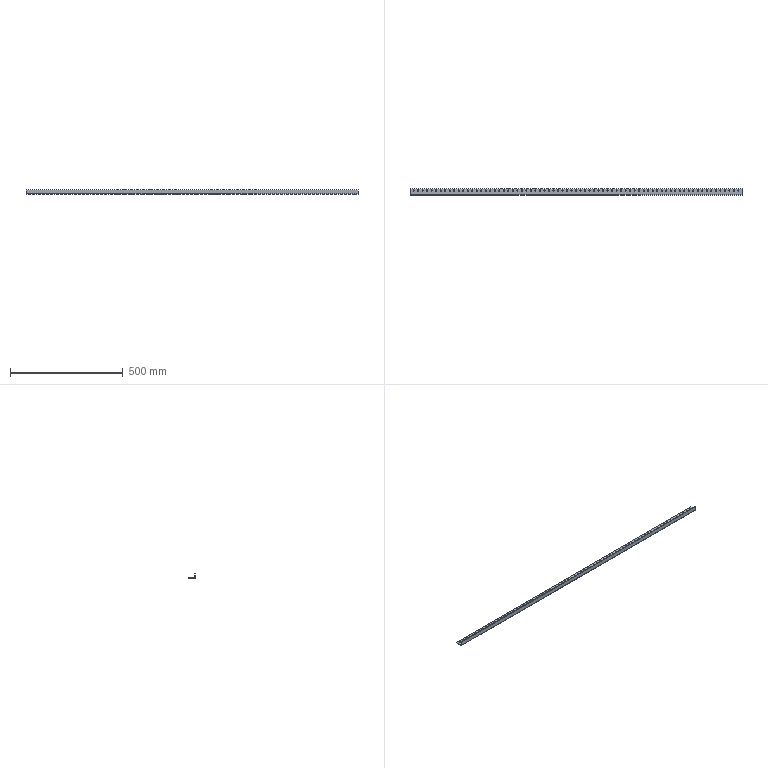Part | SolidWorks | features BaseBody 1, ICE 1, MoveFace 1 | 1 solid | 156 faces | box 1472 x 31 x 20 mm | volume 172321 mm3 | cylinder 148 | plane 8 | commonest cylinder face diameters 5.3 x146 0.2 x1 5.2 x1